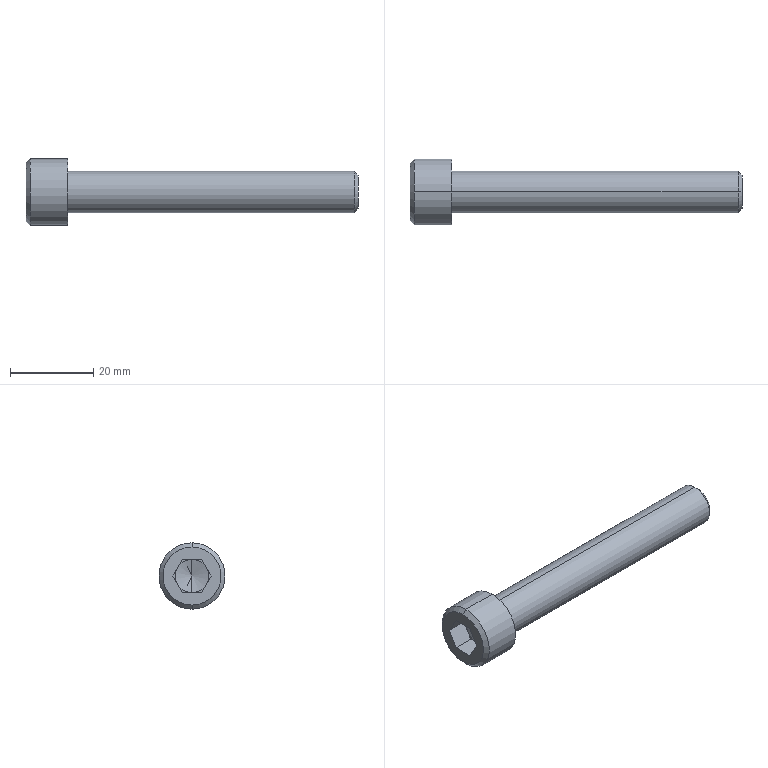Part | STEP file | CB10-70 | 1 solid | 25 faces | box 80 x 16 x 16 mm | volume 7177 mm3 | plane 15 | cone 6 | cylinder 4 | commonest cylinder face diameters 10 x2 16 x2